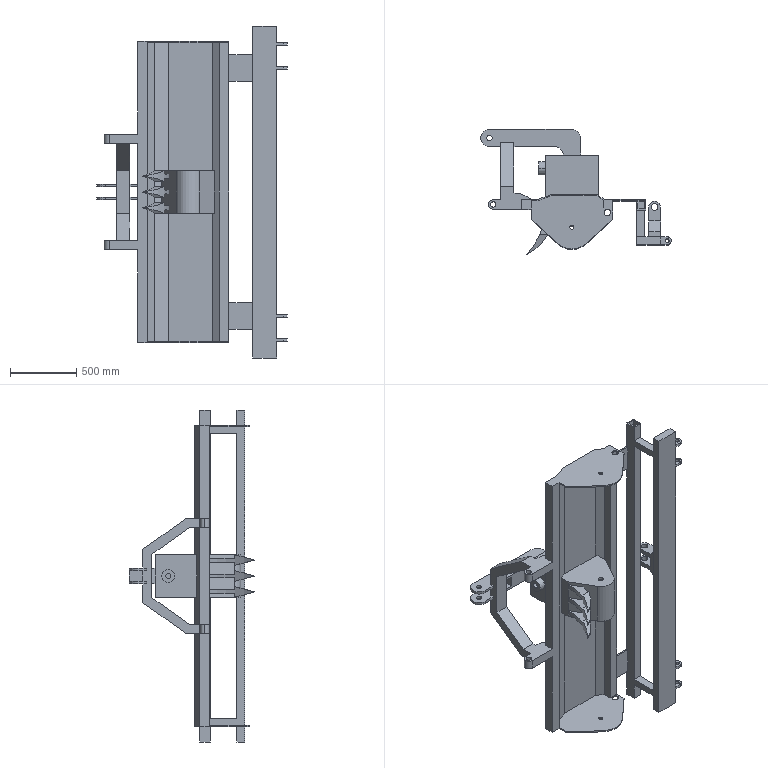Part | SolidWorks | 1 solid | 213 faces | box 1433 x 943.59 x 2500 mm | volume 127808893 mm3 | plane 147 | cylinder 66 | commonest cylinder face diameters 40 x16 30 x12 50 x8 60 x6 72 x4 700 x3